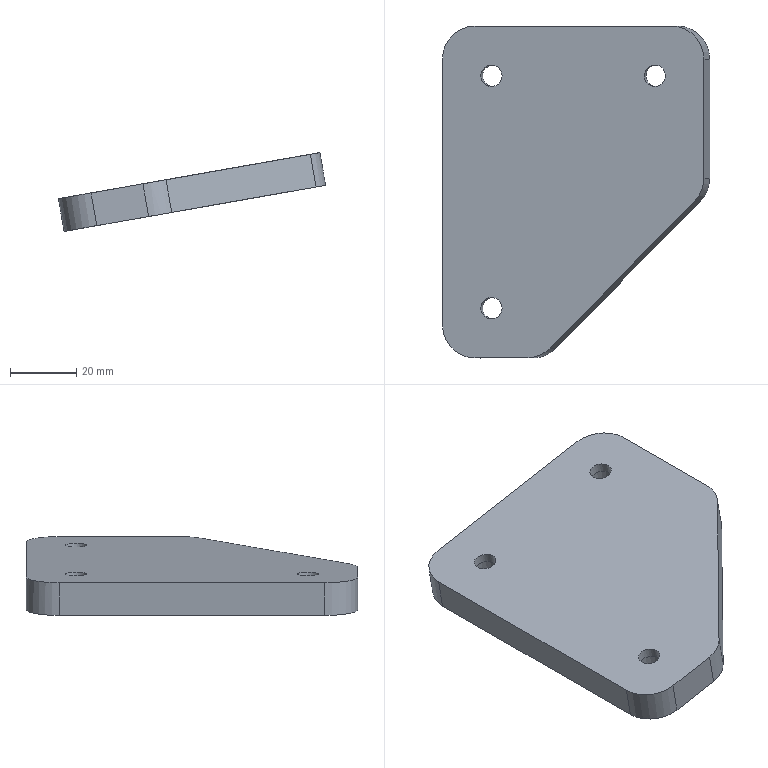Part | STEP file | solid 181 | 1 solid | 21 faces | box 80.521 x 100 x 23.74 mm | volume 64518 mm3 | cylinder 11 | plane 9 | spline 1 | commonest cylinder face diameters 20 x5 6.5 x3 11 x3